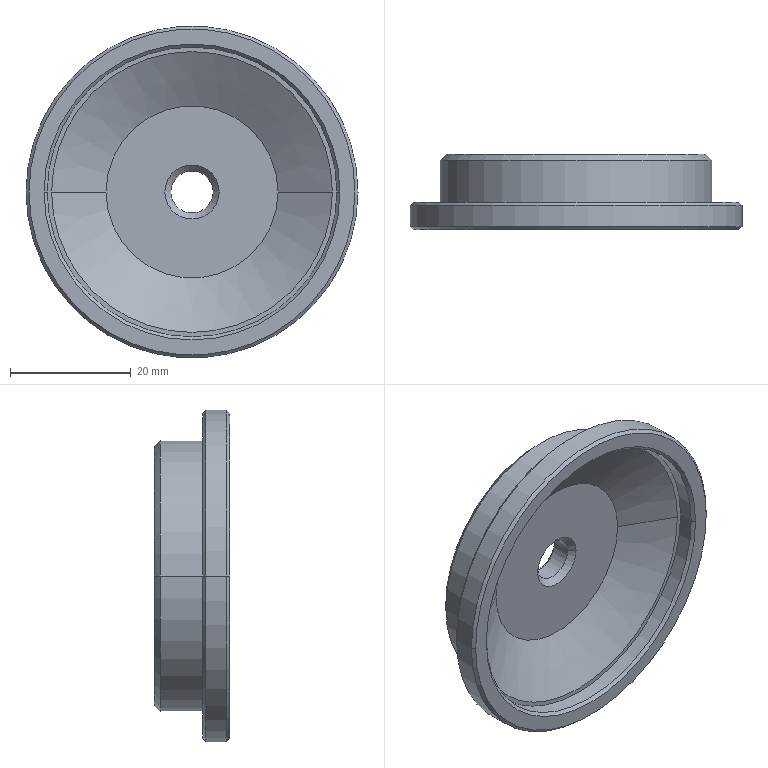Part | STEP file | 1 solid | 27 faces | box 55 x 12.5 x 55 mm | volume 12038 mm3 | cone 14 | cylinder 8 | plane 5 | commonest cylinder face diameters 7 x2 45 x2 48 x2 55 x2